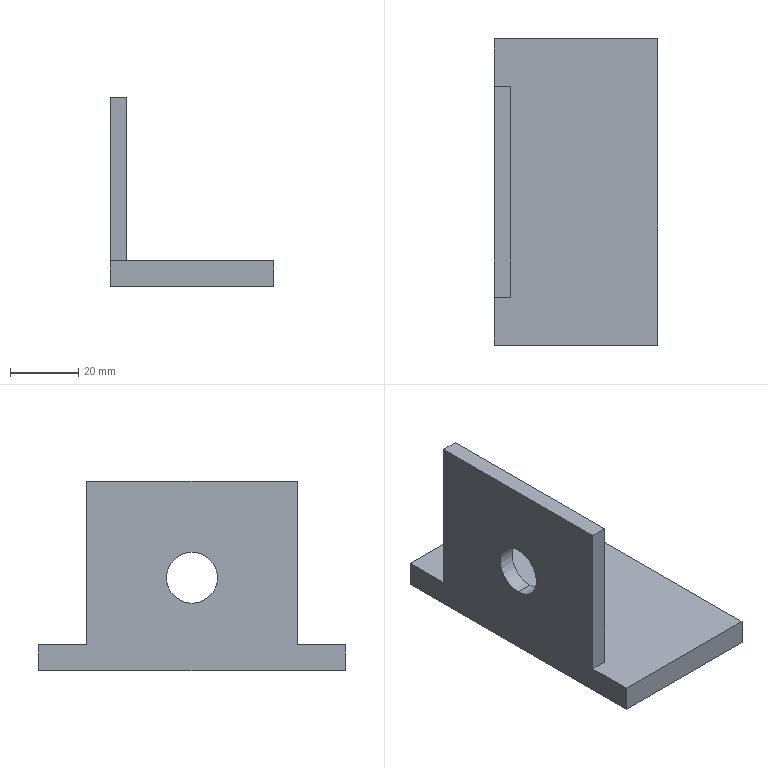Part | STEP file | 1 solid | 12 faces | box 48 x 90 x 55.597 mm | volume 46408 mm3 | plane 10 | cylinder 2 | commonest cylinder face diameters 15 x2
STEP:
#1=CARTESIAN_POINT('',(0.,0.,0.));
#2=DIRECTION('',(0.,0.,1.));
#3=DIRECTION('',(1.,0.,0.));
#4=AXIS2_PLACEMENT_3D('',#1,#2,#3);
#5=CARTESIAN_POINT('',(-595.146,553.5,112.406));
#6=VERTEX_POINT('',#5);
#7=CARTESIAN_POINT('',(-600.,553.5,112.406));
#8=VERTEX_POINT('',#7);
#9=CARTESIAN_POINT('',(-542.,553.5,112.406));
#10=DIRECTION('',(-1.,0.,0.));
#11=VECTOR('',#10,1.);
#12=LINE('',#9,#11);
#13=CARTESIAN_POINT('',(-542.,553.5,104.906));
#14=DIRECTION('',(-1.,0.,0.));
#15=DIRECTION('',(0.,0.,1.));
#16=AXIS2_PLACEMENT_3D('',#13,#14,#15);
#17=CYLINDRICAL_SURFACE('',#16,7.5);
#18=CARTESIAN_POINT('',(6.283,0.));
#19=DIRECTION('',(0.,1.));
#20=VECTOR('',#19,1.);
#21=LINE('',#18,#20);
#22=(GEOMETRIC_REPRESENTATION_CONTEXT(2)PARAMETRIC_REPRESENTATION_CONTEXT()REPRESENTATION_CONTEXT('',''));
#23=DEFINITIONAL_REPRESENTATION('',(#21),#22);
#24=PCURVE('',#17,#23);
#25=CARTESIAN_POINT('',(-542.,553.5,104.906));
#26=DIRECTION('',(-1.,0.,0.));
#27=DIRECTION('',(0.,0.,1.));
#28=AXIS2_PLACEMENT_3D('',#25,#26,#27);
#29=CYLINDRICAL_SURFACE('',#28,7.5);
#30=CARTESIAN_POINT('',(0.,0.));
#31=DIRECTION('',(0.,1.));
#32=VECTOR('',#31,1.);
#33=LINE('',#30,#32);
#34=(GEOMETRIC_REPRESENTATION_CONTEXT(2)PARAMETRIC_REPRESENTATION_CONTEXT()REPRESENTATION_CONTEXT('',''));
#35=DEFINITIONAL_REPRESENTATION('',(#33),#34);
#36=PCURVE('',#29,#35);
#37=SURFACE_CURVE('',#12,(#24,#36),.PCURVE_S1.);
#38=EDGE_CURVE('',#6,#8,#37,.T.);
#39=ORIENTED_EDGE('',*,*,#38,.T.);
#40=CARTESIAN_POINT('',(-600.,553.5,97.406));
#41=VERTEX_POINT('',#40);
#42=CARTESIAN_POINT('',(-600.,553.5,104.906));
#43=DIRECTION('',(-1.,0.,0.));
#44=DIRECTION('',(0.,0.,1.));
#45=AXIS2_PLACEMENT_3D('',#42,#43,#44);
#46=CIRCLE('',#45,7.5);
#47=CARTESIAN_POINT('',(0.,58.));
#48=DIRECTION('',(1.,0.));
#49=VECTOR('',#48,1.);
#50=LINE('',#47,#49);
#51=(GEOMETRIC_REPRESENTATION_CONTEXT(2)PARAMETRIC_REPRESENTATION_CONTEXT()REPRESENTATION_CONTEXT('',''));
#52=DEFINITIONAL_REPRESENTATION('',(#50),#51);
#53=PCURVE('',#17,#52);
#54=CARTESIAN_POINT('',(-600.,0.,133.232));
#55=DIRECTION('',(1.,0.,0.));
#56=DIRECTION('',(0.,0.,-1.));
#57=AXIS2_PLACEMENT_3D('',#54,#55,#56);
#58=PLANE('',#57);
#59=CARTESIAN_POINT('',(20.826,553.5));
#60=CARTESIAN_POINT('',(20.826,566.49));
#61=CARTESIAN_POINT('',(32.076,559.995));
#62=CARTESIAN_POINT('',(43.326,553.5));
#63=CARTESIAN_POINT('',(32.076,547.005));
#64=CARTESIAN_POINT('',(20.826,540.51));
#65=CARTESIAN_POINT('',(20.826,553.5));
#66=(BOUNDED_CURVE()B_SPLINE_CURVE(2,(#59,#60,#61,#62,#63,#64,#65),.UNSPECIFIED.,.T.,.F.)B_SPLINE_CURVE_WITH_KNOTS((1,2,2,2,2,1),(-2.094,0.,2.094,4.189,6.283,8.378),.UNSPECIFIED.)CURVE()GEOMETRIC_REPRESENTATION_ITEM()RATIONAL_B_SPLINE_CURVE((1.,0.5,1.,0.5,1.,0.5,1.))REPRESENTATION_ITEM(''));
#67=(GEOMETRIC_REPRESENTATION_CONTEXT(2)PARAMETRIC_REPRESENTATION_CONTEXT()REPRESENTATION_CONTEXT('',''));
#68=DEFINITIONAL_REPRESENTATION('',(#66),#67);
#69=PCURVE('',#58,#68);
#70=SURFACE_CURVE('',#46,(#53,#69),.PCURVE_S1.);
#71=EDGE_CURVE('',#41,#8,#70,.T.);
#72=ORIENTED_EDGE('',*,*,#71,.F.);
#73=CARTESIAN_POINT('',(-595.146,553.5,97.406));
#74=VERTEX_POINT('',#73);
#75=CARTESIAN_POINT('',(-542.,553.5,97.406));
#76=DIRECTION('',(-1.,0.,0.));
#77=VECTOR('',#76,1.);
#78=LINE('',#75,#77);
#79=CARTESIAN_POINT('',(3.142,0.));
#80=DIRECTION('',(0.,1.));
#81=VECTOR('',#80,1.);
#82=LINE('',#79,#81);
#83=(GEOMETRIC_REPRESENTATION_CONTEXT(2)PARAMETRIC_REPRESENTATION_CONTEXT()REPRESENTATION_CONTEXT('',''));
#84=DEFINITIONAL_REPRESENTATION('',(#82),#83);
#85=PCURVE('',#17,#84);
#86=CARTESIAN_POINT('',(3.142,0.));
#87=DIRECTION('',(0.,1.));
#88=VECTOR('',#87,1.);
#89=LINE('',#86,#88);
#90=(GEOMETRIC_REPRESENTATION_CONTEXT(2)PARAMETRIC_REPRESENTATION_CONTEXT()REPRESENTATION_CONTEXT('',''));
#91=DEFINITIONAL_REPRESENTATION('',(#89),#90);
#92=PCURVE('',#29,#91);
#93=SURFACE_CURVE('',#78,(#85,#92),.PCURVE_S1.);
#94=EDGE_CURVE('',#74,#41,#93,.T.);
#95=ORIENTED_EDGE('',*,*,#94,.F.);
#96=CARTESIAN_POINT('',(-595.146,553.5,104.906));
#97=DIRECTION('',(-1.,0.,0.));
#98=DIRECTION('',(0.,0.,1.));
#99=AXIS2_PLACEMENT_3D('',#96,#97,#98);
#100=CIRCLE('',#99,7.5);
#101=CARTESIAN_POINT('',(0.,53.146));
#102=DIRECTION('',(1.,0.));
#103=VECTOR('',#102,1.);
#104=LINE('',#101,#103);
#105=(GEOMETRIC_REPRESENTATION_CONTEXT(2)PARAMETRIC_REPRESENTATION_CONTEXT()REPRESENTATION_CONTEXT('',''));
#106=DEFINITIONAL_REPRESENTATION('',(#104),#105);
#107=PCURVE('',#17,#106);
#108=CARTESIAN_POINT('',(-595.146,0.,133.232));
#109=DIRECTION('',(-1.,0.,0.));
#110=DIRECTION('',(0.,0.,1.));
#111=AXIS2_PLACEMENT_3D('',#108,#109,#110);
#112=PLANE('',#111);
#113=CARTESIAN_POINT('',(-28.326,553.5));
#114=DIRECTION('',(1.,0.));
#115=AXIS2_PLACEMENT_2D('',#113,#114);
#116=CIRCLE('',#115,7.5);
#117=(GEOMETRIC_REPRESENTATION_CONTEXT(2)PARAMETRIC_REPRESENTATION_CONTEXT()REPRESENTATION_CONTEXT('',''));
#118=DEFINITIONAL_REPRESENTATION('',(#116),#117);
#119=PCURVE('',#112,#118);
#120=SURFACE_CURVE('',#100,(#107,#119),.PCURVE_S1.);
#121=EDGE_CURVE('',#74,#6,#120,.T.);
#122=ORIENTED_EDGE('',*,*,#121,.T.);
#123=EDGE_LOOP('',(#39,#72,#95,#122));
#124=FACE_BOUND('',#123,.F.);
#125=ADVANCED_FACE('',(#124),#17,.F.);
#126=CARTESIAN_POINT('',(-600.,553.5,104.906));
#127=DIRECTION('',(-1.,0.,0.));
#128=DIRECTION('',(0.,0.,1.));
#129=AXIS2_PLACEMENT_3D('',#126,#127,#128);
#130=CIRCLE('',#129,7.5);
#131=CARTESIAN_POINT('',(20.826,553.5));
#132=CARTESIAN_POINT('',(20.826,566.49));
#133=CARTESIAN_POINT('',(32.076,559.995));
#134=CARTESIAN_POINT('',(43.326,553.5));
#135=CARTESIAN_POINT('',(32.076,547.005));
#136=CARTESIAN_POINT('',(20.826,540.51));
#137=CARTESIAN_POINT('',(20.826,553.5));
#138=(BOUNDED_CURVE()B_SPLINE_CURVE(2,(#131,#132,#133,#134,#135,#136,#137),.UNSPECIFIED.,.T.,.F.)B_SPLINE_CURVE_WITH_KNOTS((1,2,2,2,2,1),(-2.094,0.,2.094,4.189,6.283,8.378),.UNSPECIFIED.)CURVE()GEOMETRIC_REPRESENTATION_ITEM()RATIONAL_B_SPLINE_CURVE((1.,0.5,1.,0.5,1.,0.5,1.))REPRESENTATION_ITEM(''));
#139=(GEOMETRIC_REPRESENTATION_CONTEXT(2)PARAMETRIC_REPRESENTATION_CONTEXT()REPRESENTATION_CONTEXT('',''));
#140=DEFINITIONAL_REPRESENTATION('',(#138),#139);
#141=PCURVE('',#58,#140);
#142=CARTESIAN_POINT('',(0.,58.));
#143=DIRECTION('',(1.,0.));
#144=VECTOR('',#143,1.);
#145=LINE('',#142,#144);
#146=(GEOMETRIC_REPRESENTATION_CONTEXT(2)PARAMETRIC_REPRESENTATION_CONTEXT()REPRESENTATION_CONTEXT('',''));
#147=DEFINITIONAL_REPRESENTATION('',(#145),#146);
#148=PCURVE('',#29,#147);
#149=SURFACE_CURVE('',#130,(#141,#148),.PCURVE_S1.);
#150=EDGE_CURVE('',#8,#41,#149,.T.);
#151=ORIENTED_EDGE('',*,*,#150,.F.);
#152=ORIENTED_EDGE('',*,*,#71,.F.);
#153=EDGE_LOOP('',(#151,#152));
#154=FACE_BOUND('',#153,.T.);
#155=CARTESIAN_POINT('',(-600.,584.5,133.232));
#156=VERTEX_POINT('',#155);
#157=CARTESIAN_POINT('',(-600.,522.5,133.232));
#158=VERTEX_POINT('',#157);
#159=CARTESIAN_POINT('',(-600.,0.,133.232));
#160=DIRECTION('',(0.,-1.,0.));
#161=VECTOR('',#160,1.);
#162=LINE('',#159,#161);
#163=CARTESIAN_POINT('',(0.,0.));
#164=DIRECTION('',(0.,-1.));
#165=VECTOR('',#164,1.);
#166=LINE('',#163,#165);
#167=(GEOMETRIC_REPRESENTATION_CONTEXT(2)PARAMETRIC_REPRESENTATION_CONTEXT()REPRESENTATION_CONTEXT('',''));
#168=DEFINITIONAL_REPRESENTATION('',(#166),#167);
#169=PCURVE('',#58,#168);
#170=CARTESIAN_POINT('',(0.,0.,133.232));
#171=DIRECTION('',(0.,0.,1.));
#172=DIRECTION('',(1.,0.,0.));
#173=AXIS2_PLACEMENT_3D('',#170,#171,#172);
#174=PLANE('',#173);
#175=CARTESIAN_POINT('',(-600.,0.));
#176=DIRECTION('',(0.,-1.));
#177=VECTOR('',#176,1.);
#178=LINE('',#175,#177);
#179=(GEOMETRIC_REPRESENTATION_CONTEXT(2)PARAMETRIC_REPRESENTATION_CONTEXT()REPRESENTATION_CONTEXT('',''));
#180=DEFINITIONAL_REPRESENTATION('',(#178),#179);
#181=PCURVE('',#174,#180);
#182=SURFACE_CURVE('',#162,(#169,#181),.PCURVE_S1.);
#183=EDGE_CURVE('',#156,#158,#182,.T.);
#184=ORIENTED_EDGE('',*,*,#183,.F.);
#185=CARTESIAN_POINT('',(-600.,584.5,85.232));
#186=VERTEX_POINT('',#185);
#187=CARTESIAN_POINT('',(-600.,584.5,133.232));
#188=DIRECTION('',(0.,0.,-1.));
#189=VECTOR('',#188,1.);
#190=LINE('',#187,#189);
#191=CARTESIAN_POINT('',(0.,584.5));
#192=DIRECTION('',(1.,0.));
#193=VECTOR('',#192,1.);
#194=LINE('',#191,#193);
#195=(GEOMETRIC_REPRESENTATION_CONTEXT(2)PARAMETRIC_REPRESENTATION_CONTEXT()REPRESENTATION_CONTEXT('',''));
#196=DEFINITIONAL_REPRESENTATION('',(#194),#195);
#197=PCURVE('',#58,#196);
#198=CARTESIAN_POINT('',(-648.717,584.5,133.232));
#199=DIRECTION('',(0.,1.,0.));
#200=DIRECTION('',(0.,0.,1.));
#201=AXIS2_PLACEMENT_3D('',#198,#199,#200);
#202=PLANE('',#201);
#203=CARTESIAN_POINT('',(0.,48.717));
#204=DIRECTION('',(-1.,0.));
#205=VECTOR('',#204,1.);
#206=LINE('',#203,#205);
#207=(GEOMETRIC_REPRESENTATION_CONTEXT(2)PARAMETRIC_REPRESENTATION_CONTEXT()REPRESENTATION_CONTEXT('',''));
#208=DEFINITIONAL_REPRESENTATION('',(#206),#207);
#209=PCURVE('',#202,#208);
#210=SURFACE_CURVE('',#190,(#197,#209),.PCURVE_S1.);
#211=EDGE_CURVE('',#156,#186,#210,.T.);
#212=ORIENTED_EDGE('',*,*,#211,.T.);
#213=CARTESIAN_POINT('',(-600.,598.5,85.232));
#214=VERTEX_POINT('',#213);
#215=CARTESIAN_POINT('',(-600.,0.,85.232));
#216=DIRECTION('',(0.,1.,0.));
#217=VECTOR('',#216,1.);
#218=LINE('',#215,#217);
#219=CARTESIAN_POINT('',(48.,0.));
#220=DIRECTION('',(0.,1.));
#221=VECTOR('',#220,1.);
#222=LINE('',#219,#221);
#223=(GEOMETRIC_REPRESENTATION_CONTEXT(2)PARAMETRIC_REPRESENTATION_CONTEXT()REPRESENTATION_CONTEXT('',''));
#224=DEFINITIONAL_REPRESENTATION('',(#222),#223);
#225=PCURVE('',#58,#224);
#226=CARTESIAN_POINT('',(-552.,0.,85.232));
#227=DIRECTION('',(0.,0.,1.));
#228=DIRECTION('',(1.,0.,0.));
#229=AXIS2_PLACEMENT_3D('',#226,#227,#228);
#230=PLANE('',#229);
#231=CARTESIAN_POINT('',(-48.,0.));
#232=DIRECTION('',(0.,1.));
#233=VECTOR('',#232,1.);
#234=LINE('',#231,#233);
#235=(GEOMETRIC_REPRESENTATION_CONTEXT(2)PARAMETRIC_REPRESENTATION_CONTEXT()REPRESENTATION_CONTEXT('',''));
#236=DEFINITIONAL_REPRESENTATION('',(#234),#235);
#237=PCURVE('',#230,#236);
#238=SURFACE_CURVE('',#218,(#225,#237),.PCURVE_S1.);
#239=EDGE_CURVE('',#186,#214,#238,.T.);
#240=ORIENTED_EDGE('',*,*,#239,.T.);
#241=CARTESIAN_POINT('',(-600.,598.5,77.635));
#242=VERTEX_POINT('',#241);
#243=CARTESIAN_POINT('',(-600.,598.5,0.));
#244=DIRECTION('',(0.,0.,1.));
#245=VECTOR('',#244,1.);
#246=LINE('',#243,#245);
#247=CARTESIAN_POINT('',(133.232,598.5));
#248=DIRECTION('',(-1.,0.));
#249=VECTOR('',#248,1.);
#250=LINE('',#247,#249);
#251=(GEOMETRIC_REPRESENTATION_CONTEXT(2)PARAMETRIC_REPRESENTATION_CONTEXT()REPRESENTATION_CONTEXT('',''));
#252=DEFINITIONAL_REPRESENTATION('',(#250),#251);
#253=PCURVE('',#58,#252);
#254=CARTESIAN_POINT('',(-552.,598.5,0.));
#255=DIRECTION('',(0.,-1.,0.));
#256=DIRECTION('',(0.,0.,-1.));
#257=AXIS2_PLACEMENT_3D('',#254,#255,#256);
#258=PLANE('',#257);
#259=CARTESIAN_POINT('',(0.,-48.));
#260=DIRECTION('',(-1.,0.));
#261=VECTOR('',#260,1.);
#262=LINE('',#259,#261);
#263=(GEOMETRIC_REPRESENTATION_CONTEXT(2)PARAMETRIC_REPRESENTATION_CONTEXT()REPRESENTATION_CONTEXT('',''));
#264=DEFINITIONAL_REPRESENTATION('',(#262),#263);
#265=PCURVE('',#258,#264);
#266=SURFACE_CURVE('',#246,(#253,#265),.PCURVE_S1.);
#267=EDGE_CURVE('',#242,#214,#266,.T.);
#268=ORIENTED_EDGE('',*,*,#267,.F.);
#269=CARTESIAN_POINT('',(-600.,508.5,77.635));
#270=VERTEX_POINT('',#269);
#271=CARTESIAN_POINT('',(-600.,0.,77.635));
#272=DIRECTION('',(0.,1.,0.));
#273=VECTOR('',#272,1.);
#274=LINE('',#271,#273);
#275=CARTESIAN_POINT('',(55.597,0.));
#276=DIRECTION('',(0.,1.));
#277=VECTOR('',#276,1.);
#278=LINE('',#275,#277);
#279=(GEOMETRIC_REPRESENTATION_CONTEXT(2)PARAMETRIC_REPRESENTATION_CONTEXT()REPRESENTATION_CONTEXT('',''));
#280=DEFINITIONAL_REPRESENTATION('',(#278),#279);
#281=PCURVE('',#58,#280);
#282=CARTESIAN_POINT('',(-552.,0.,77.635));
#283=DIRECTION('',(0.,0.,1.));
#284=DIRECTION('',(1.,0.,0.));
#285=AXIS2_PLACEMENT_3D('',#282,#283,#284);
#286=PLANE('',#285);
#287=CARTESIAN_POINT('',(-48.,0.));
#288=DIRECTION('',(0.,1.));
#289=VECTOR('',#288,1.);
#290=LINE('',#287,#289);
#291=(GEOMETRIC_REPRESENTATION_CONTEXT(2)PARAMETRIC_REPRESENTATION_CONTEXT()REPRESENTATION_CONTEXT('',''));
#292=DEFINITIONAL_REPRESENTATION('',(#290),#291);
#293=PCURVE('',#286,#292);
#294=SURFACE_CURVE('',#274,(#281,#293),.PCURVE_S1.);
#295=EDGE_CURVE('',#270,#242,#294,.T.);
#296=ORIENTED_EDGE('',*,*,#295,.F.);
#297=CARTESIAN_POINT('',(-600.,508.5,85.232));
#298=VERTEX_POINT('',#297);
#299=CARTESIAN_POINT('',(-600.,508.5,0.));
#300=DIRECTION('',(0.,0.,1.));
#301=VECTOR('',#300,1.);
#302=LINE('',#299,#301);
#303=CARTESIAN_POINT('',(133.232,508.5));
#304=DIRECTION('',(-1.,0.));
#305=VECTOR('',#304,1.);
#306=LINE('',#303,#305);
#307=(GEOMETRIC_REPRESENTATION_CONTEXT(2)PARAMETRIC_REPRESENTATION_CONTEXT()REPRESENTATION_CONTEXT('',''));
#308=DEFINITIONAL_REPRESENTATION('',(#306),#307);
#309=PCURVE('',#58,#308);
#310=CARTESIAN_POINT('',(-552.,508.5,0.));
#311=DIRECTION('',(0.,-1.,0.));
#312=DIRECTION('',(0.,0.,-1.));
#313=AXIS2_PLACEMENT_3D('',#310,#311,#312);
#314=PLANE('',#313);
#315=CARTESIAN_POINT('',(0.,-48.));
#316=DIRECTION('',(-1.,0.));
#317=VECTOR('',#316,1.);
#318=LINE('',#315,#317);
#319=(GEOMETRIC_REPRESENTATION_CONTEXT(2)PARAMETRIC_REPRESENTATION_CONTEXT()REPRESENTATION_CONTEXT('',''));
#320=DEFINITIONAL_REPRESENTATION('',(#318),#319);
#321=PCURVE('',#314,#320);
#322=SURFACE_CURVE('',#302,(#309,#321),.PCURVE_S1.);
#323=EDGE_CURVE('',#270,#298,#322,.T.);
#324=ORIENTED_EDGE('',*,*,#323,.T.);
#325=CARTESIAN_POINT('',(-600.,522.5,85.232));
#326=VERTEX_POINT('',#325);
#327=CARTESIAN_POINT('',(-600.,0.,85.232));
#328=DIRECTION('',(0.,1.,0.));
#329=VECTOR('',#328,1.);
#330=LINE('',#327,#329);
#331=CARTESIAN_POINT('',(48.,0.));
#332=DIRECTION('',(0.,1.));
#333=VECTOR('',#332,1.);
#334=LINE('',#331,#333);
#335=(GEOMETRIC_REPRESENTATION_CONTEXT(2)PARAMETRIC_REPRESENTATION_CONTEXT()REPRESENTATION_CONTEXT('',''));
#336=DEFINITIONAL_REPRESENTATION('',(#334),#335);
#337=PCURVE('',#58,#336);
#338=CARTESIAN_POINT('',(-48.,0.));
#339=DIRECTION('',(0.,1.));
#340=VECTOR('',#339,1.);
#341=LINE('',#338,#340);
#342=(GEOMETRIC_REPRESENTATION_CONTEXT(2)PARAMETRIC_REPRESENTATION_CONTEXT()REPRESENTATION_CONTEXT('',''));
#343=DEFINITIONAL_REPRESENTATION('',(#341),#342);
#344=PCURVE('',#230,#343);
#345=SURFACE_CURVE('',#330,(#337,#344),.PCURVE_S1.);
#346=EDGE_CURVE('',#298,#326,#345,.T.);
#347=ORIENTED_EDGE('',*,*,#346,.T.);
#348=CARTESIAN_POINT('',(-600.,522.5,133.232));
#349=DIRECTION('',(0.,0.,1.));
#350=VECTOR('',#349,1.);
#351=LINE('',#348,#350);
#352=CARTESIAN_POINT('',(0.,522.5));
#353=DIRECTION('',(-1.,0.));
#354=VECTOR('',#353,1.);
#355=LINE('',#352,#354);
#356=(GEOMETRIC_REPRESENTATION_CONTEXT(2)PARAMETRIC_REPRESENTATION_CONTEXT()REPRESENTATION_CONTEXT('',''));
#357=DEFINITIONAL_REPRESENTATION('',(#355),#356);
#358=PCURVE('',#58,#357);
#359=CARTESIAN_POINT('',(-648.717,522.5,133.232));
#360=DIRECTION('',(0.,-1.,0.));
#361=DIRECTION('',(0.,0.,-1.));
#362=AXIS2_PLACEMENT_3D('',#359,#360,#361);
#363=PLANE('',#362);
#364=CARTESIAN_POINT('',(0.,48.717));
#365=DIRECTION('',(-1.,0.));
#366=VECTOR('',#365,1.);
#367=LINE('',#364,#366);
#368=(GEOMETRIC_REPRESENTATION_CONTEXT(2)PARAMETRIC_REPRESENTATION_CONTEXT()REPRESENTATION_CONTEXT('',''));
#369=DEFINITIONAL_REPRESENTATION('',(#367),#368);
#370=PCURVE('',#363,#369);
#371=SURFACE_CURVE('',#351,(#358,#370),.PCURVE_S1.);
#372=EDGE_CURVE('',#326,#158,#371,.T.);
#373=ORIENTED_EDGE('',*,*,#372,.T.);
#374=EDGE_LOOP('',(#184,#212,#240,#268,#296,#324,#347,#373));
#375=FACE_BOUND('',#374,.T.);
#376=ADVANCED_FACE('',(#154,#375),#58,.F.);
#377=CARTESIAN_POINT('',(-595.146,553.5,104.906));
#378=DIRECTION('',(-1.,0.,0.));
#379=DIRECTION('',(0.,0.,1.));
#380=AXIS2_PLACEMENT_3D('',#377,#378,#379);
#381=CIRCLE('',#380,7.5);
#382=CARTESIAN_POINT('',(-28.326,553.5));
#383=DIRECTION('',(1.,0.));
#384=AXIS2_PLACEMENT_2D('',#382,#383);
#385=CIRCLE('',#384,7.5);
#386=(GEOMETRIC_REPRESENTATION_CONTEXT(2)PARAMETRIC_REPRESENTATION_CONTEXT()REPRESENTATION_CONTEXT('',''));
#387=DEFINITIONAL_REPRESENTATION('',(#385),#386);
#388=PCURVE('',#112,#387);
#389=CARTESIAN_POINT('',(0.,53.146));
#390=DIRECTION('',(1.,0.));
#391=VECTOR('',#390,1.);
#392=LINE('',#389,#391);
#393=(GEOMETRIC_REPRESENTATION_CONTEXT(2)PARAMETRIC_REPRESENTATION_CONTEXT()REPRESENTATION_CONTEXT('',''));
#394=DEFINITIONAL_REPRESENTATION('',(#392),#393);
#395=PCURVE('',#29,#394);
#396=SURFACE_CURVE('',#381,(#388,#395),.PCURVE_S1.);
#397=EDGE_CURVE('',#6,#74,#396,.T.);
#398=ORIENTED_EDGE('',*,*,#397,.T.);
#399=ORIENTED_EDGE('',*,*,#121,.T.);
#400=EDGE_LOOP('',(#398,#399));
#401=FACE_BOUND('',#400,.T.);
#402=CARTESIAN_POINT('',(-595.146,522.5,85.232));
#403=VERTEX_POINT('',#402);
#404=CARTESIAN_POINT('',(-595.146,584.5,85.232));
#405=VERTEX_POINT('',#404);
#406=CARTESIAN_POINT('',(-595.146,0.,85.232));
#407=DIRECTION('',(0.,1.,0.));
#408=VECTOR('',#407,1.);
#409=LINE('',#406,#408);
#410=CARTESIAN_POINT('',(-48.,0.));
#411=DIRECTION('',(0.,1.));
#412=VECTOR('',#411,1.);
#413=LINE('',#410,#412);
#414=(GEOMETRIC_REPRESENTATION_CONTEXT(2)PARAMETRIC_REPRESENTATION_CONTEXT()REPRESENTATION_CONTEXT('',''));
#415=DEFINITIONAL_REPRESENTATION('',(#413),#414);
#416=PCURVE('',#112,#415);
#417=CARTESIAN_POINT('',(-43.146,0.));
#418=DIRECTION('',(0.,1.));
#419=VECTOR('',#418,1.);
#420=LINE('',#417,#419);
#421=(GEOMETRIC_REPRESENTATION_CONTEXT(2)PARAMETRIC_REPRESENTATION_CONTEXT()REPRESENTATION_CONTEXT('',''));
#422=DEFINITIONAL_REPRESENTATION('',(#420),#421);
#423=PCURVE('',#230,#422);
#424=SURFACE_CURVE('',#409,(#416,#423),.PCURVE_S1.);
#425=EDGE_CURVE('',#403,#405,#424,.T.);
#426=ORIENTED_EDGE('',*,*,#425,.T.);
#427=CARTESIAN_POINT('',(-595.146,584.5,133.232));
#428=VERTEX_POINT('',#427);
#429=CARTESIAN_POINT('',(-595.146,584.5,133.232));
#430=DIRECTION('',(0.,0.,1.));
#431=VECTOR('',#430,1.);
#432=LINE('',#429,#431);
#433=CARTESIAN_POINT('',(0.,584.5));
#434=DIRECTION('',(1.,0.));
#435=VECTOR('',#434,1.);
#436=LINE('',#433,#435);
#437=(GEOMETRIC_REPRESENTATION_CONTEXT(2)PARAMETRIC_REPRESENTATION_CONTEXT()REPRESENTATION_CONTEXT('',''));
#438=DEFINITIONAL_REPRESENTATION('',(#436),#437);
#439=PCURVE('',#112,#438);
#440=CARTESIAN_POINT('',(0.,53.571));
#441=DIRECTION('',(1.,0.));
#442=VECTOR('',#441,1.);
#443=LINE('',#440,#442);
#444=(GEOMETRIC_REPRESENTATION_CONTEXT(2)PARAMETRIC_REPRESENTATION_CONTEXT()REPRESENTATION_CONTEXT('',''));
#445=DEFINITIONAL_REPRESENTATION('',(#443),#444);
#446=PCURVE('',#202,#445);
#447=SURFACE_CURVE('',#432,(#439,#446),.PCURVE_S1.);
#448=EDGE_CURVE('',#405,#428,#447,.T.);
#449=ORIENTED_EDGE('',*,*,#448,.T.);
#450=CARTESIAN_POINT('',(-595.146,522.5,133.232));
#451=VERTEX_POINT('',#450);
#452=CARTESIAN_POINT('',(-595.146,0.,133.232));
#453=DIRECTION('',(0.,1.,0.));
#454=VECTOR('',#453,1.);
#455=LINE('',#452,#454);
#456=CARTESIAN_POINT('',(0.,0.));
#457=DIRECTION('',(0.,1.));
#458=VECTOR('',#457,1.);
#459=LINE('',#456,#458);
#460=(GEOMETRIC_REPRESENTATION_CONTEXT(2)PARAMETRIC_REPRESENTATION_CONTEXT()REPRESENTATION_CONTEXT('',''));
#461=DEFINITIONAL_REPRESENTATION('',(#459),#460);
#462=PCURVE('',#112,#461);
#463=CARTESIAN_POINT('',(-595.146,0.));
#464=DIRECTION('',(0.,1.));
#465=VECTOR('',#464,1.);
#466=LINE('',#463,#465);
#467=(GEOMETRIC_REPRESENTATION_CONTEXT(2)PARAMETRIC_REPRESENTATION_CONTEXT()REPRESENTATION_CONTEXT('',''));
#468=DEFINITIONAL_REPRESENTATION('',(#466),#467);
#469=PCURVE('',#174,#468);
#470=SURFACE_CURVE('',#455,(#462,#469),.PCURVE_S1.);
#471=EDGE_CURVE('',#451,#428,#470,.T.);
#472=ORIENTED_EDGE('',*,*,#471,.F.);
#473=CARTESIAN_POINT('',(-595.146,522.5,133.232));
#474=DIRECTION('',(0.,0.,-1.));
#475=VECTOR('',#474,1.);
#476=LINE('',#473,#475);
#477=CARTESIAN_POINT('',(0.,522.5));
#478=DIRECTION('',(-1.,0.));
#479=VECTOR('',#478,1.);
#480=LINE('',#477,#479);
#481=(GEOMETRIC_REPRESENTATION_CONTEXT(2)PARAMETRIC_REPRESENTATION_CONTEXT()REPRESENTATION_CONTEXT('',''));
#482=DEFINITIONAL_REPRESENTATION('',(#480),#481);
#483=PCURVE('',#112,#482);
#484=CARTESIAN_POINT('',(0.,53.571));
#485=DIRECTION('',(1.,0.));
#486=VECTOR('',#485,1.);
#487=LINE('',#484,#486);
#488=(GEOMETRIC_REPRESENTATION_CONTEXT(2)PARAMETRIC_REPRESENTATION_CONTEXT()REPRESENTATION_CONTEXT('',''));
#489=DEFINITIONAL_REPRESENTATION('',(#487),#488);
#490=PCURVE('',#363,#489);
#491=SURFACE_CURVE('',#476,(#483,#490),.PCURVE_S1.);
#492=EDGE_CURVE('',#451,#403,#491,.T.);
#493=ORIENTED_EDGE('',*,*,#492,.T.);
#494=EDGE_LOOP('',(#426,#449,#472,#493));
#495=FACE_BOUND('',#494,.T.);
#496=ADVANCED_FACE('',(#401,#495),#112,.F.);
#497=ORIENTED_EDGE('',*,*,#183,.T.);
#498=CARTESIAN_POINT('',(-648.717,522.5,133.232));
#499=DIRECTION('',(1.,0.,0.));
#500=VECTOR('',#499,1.);
#501=LINE('',#498,#500);
#502=CARTESIAN_POINT('',(-648.717,522.5));
#503=DIRECTION('',(1.,0.));
#504=VECTOR('',#503,1.);
#505=LINE('',#502,#504);
#506=(GEOMETRIC_REPRESENTATION_CONTEXT(2)PARAMETRIC_REPRESENTATION_CONTEXT()REPRESENTATION_CONTEXT('',''));
#507=DEFINITIONAL_REPRESENTATION('',(#505),#506);
#508=PCURVE('',#174,#507);
#509=CARTESIAN_POINT('',(0.,0.));
#510=DIRECTION('',(0.,1.));
#511=VECTOR('',#510,1.);
#512=LINE('',#509,#511);
#513=(GEOMETRIC_REPRESENTATION_CONTEXT(2)PARAMETRIC_REPRESENTATION_CONTEXT()REPRESENTATION_CONTEXT('',''));
#514=DEFINITIONAL_REPRESENTATION('',(#512),#513);
#515=PCURVE('',#363,#514);
#516=SURFACE_CURVE('',#501,(#508,#515),.PCURVE_S1.);
#517=EDGE_CURVE('',#158,#451,#516,.T.);
#518=ORIENTED_EDGE('',*,*,#517,.T.);
#519=ORIENTED_EDGE('',*,*,#471,.T.);
#520=CARTESIAN_POINT('',(-648.717,584.5,133.232));
#521=DIRECTION('',(1.,0.,0.));
#522=VECTOR('',#521,1.);
#523=LINE('',#520,#522);
#524=CARTESIAN_POINT('',(-648.717,584.5));
#525=DIRECTION('',(1.,0.));
#526=VECTOR('',#525,1.);
#527=LINE('',#524,#526);
#528=(GEOMETRIC_REPRESENTATION_CONTEXT(2)PARAMETRIC_REPRESENTATION_CONTEXT()REPRESENTATION_CONTEXT('',''));
#529=DEFINITIONAL_REPRESENTATION('',(#527),#528);
#530=PCURVE('',#174,#529);
#531=CARTESIAN_POINT('',(0.,0.));
#532=DIRECTION('',(0.,1.));
#533=VECTOR('',#532,1.);
#534=LINE('',#531,#533);
#535=(GEOMETRIC_REPRESENTATION_CONTEXT(2)PARAMETRIC_REPRESENTATION_CONTEXT()REPRESENTATION_CONTEXT('',''));
#536=DEFINITIONAL_REPRESENTATION('',(#534),#535);
#537=PCURVE('',#202,#536);
#538=SURFACE_CURVE('',#523,(#530,#537),.PCURVE_S1.);
#539=EDGE_CURVE('',#156,#428,#538,.T.);
#540=ORIENTED_EDGE('',*,*,#539,.F.);
#541=EDGE_LOOP('',(#497,#518,#519,#540));
#542=FACE_BOUND('',#541,.T.);
#543=ADVANCED_FACE('',(#542),#174,.T.);
#544=ORIENTED_EDGE('',*,*,#295,.T.);
#545=CARTESIAN_POINT('',(-552.,598.5,77.635));
#546=VERTEX_POINT('',#545);
#547=CARTESIAN_POINT('',(-552.,598.5,77.635));
#548=DIRECTION('',(-1.,0.,0.));
#549=VECTOR('',#548,1.);
#550=LINE('',#547,#549);
#551=CARTESIAN_POINT('',(0.,598.5));
#552=DIRECTION('',(-1.,0.));
#553=VECTOR('',#552,1.);
#554=LINE('',#551,#553);
#555=(GEOMETRIC_REPRESENTATION_CONTEXT(2)PARAMETRIC_REPRESENTATION_CONTEXT()REPRESENTATION_CONTEXT('',''));
#556=DEFINITIONAL_REPRESENTATION('',(#554),#555);
#557=PCURVE('',#286,#556);
#558=CARTESIAN_POINT('',(-77.635,0.));
#559=DIRECTION('',(0.,-1.));
#560=VECTOR('',#559,1.);
#561=LINE('',#558,#560);
#562=(GEOMETRIC_REPRESENTATION_CONTEXT(2)PARAMETRIC_REPRESENTATION_CONTEXT()REPRESENTATION_CONTEXT('',''));
#563=DEFINITIONAL_REPRESENTATION('',(#561),#562);
#564=PCURVE('',#258,#563);
#565=SURFACE_CURVE('',#550,(#557,#564),.PCURVE_S1.);
#566=EDGE_CURVE('',#546,#242,#565,.T.);
#567=ORIENTED_EDGE('',*,*,#566,.F.);
#568=CARTESIAN_POINT('',(-552.,508.5,77.635));
#569=VERTEX_POINT('',#568);
#570=CARTESIAN_POINT('',(-552.,0.,77.635));
#571=DIRECTION('',(0.,1.,0.));
#572=VECTOR('',#571,1.);
#573=LINE('',#570,#572);
#574=CARTESIAN_POINT('',(0.,0.));
#575=DIRECTION('',(0.,1.));
#576=VECTOR('',#575,1.);
#577=LINE('',#574,#576);
#578=(GEOMETRIC_REPRESENTATION_CONTEXT(2)PARAMETRIC_REPRESENTATION_CONTEXT()REPRESENTATION_CONTEXT('',''));
#579=DEFINITIONAL_REPRESENTATION('',(#577),#578);
#580=PCURVE('',#286,#579);
#581=CARTESIAN_POINT('',(-552.,0.,0.));
#582=DIRECTION('',(-1.,0.,0.));
#583=DIRECTION('',(0.,0.,1.));
#584=AXIS2_PLACEMENT_3D('',#581,#582,#583);
#585=PLANE('',#584);
#586=CARTESIAN_POINT('',(77.635,0.));
#587=DIRECTION('',(0.,1.));
#588=VECTOR('',#587,1.);
#589=LINE('',#586,#588);
#590=(GEOMETRIC_REPRESENTATION_CONTEXT(2)PARAMETRIC_REPRESENTATION_CONTEXT()REPRESENTATION_CONTEXT('',''));
#591=DEFINITIONAL_REPRESENTATION('',(#589),#590);
#592=PCURVE('',#585,#591);
#593=SURFACE_CURVE('',#573,(#580,#592),.PCURVE_S1.);
#594=EDGE_CURVE('',#569,#546,#593,.T.);
#595=ORIENTED_EDGE('',*,*,#594,.F.);
#596=CARTESIAN_POINT('',(-552.,508.5,77.635));
#597=DIRECTION('',(-1.,0.,0.));
#598=VECTOR('',#597,1.);
#599=LINE('',#596,#598);
#600=CARTESIAN_POINT('',(0.,508.5));
#601=DIRECTION('',(-1.,0.));
#602=VECTOR('',#601,1.);
#603=LINE('',#600,#602);
#604=(GEOMETRIC_REPRESENTATION_CONTEXT(2)PARAMETRIC_REPRESENTATION_CONTEXT()REPRESENTATION_CONTEXT('',''));
#605=DEFINITIONAL_REPRESENTATION('',(#603),#604);
#606=PCURVE('',#286,#605);
#607=CARTESIAN_POINT('',(-77.635,0.));
#608=DIRECTION('',(0.,-1.));
#609=VECTOR('',#608,1.);
#610=LINE('',#607,#609);
#611=(GEOMETRIC_REPRESENTATION_CONTEXT(2)PARAMETRIC_REPRESENTATION_CONTEXT()REPRESENTATION_CONTEXT('',''));
#612=DEFINITIONAL_REPRESENTATION('',(#610),#611);
#613=PCURVE('',#314,#612);
#614=SURFACE_CURVE('',#599,(#606,#613),.PCURVE_S1.);
#615=EDGE_CURVE('',#569,#270,#614,.T.);
#616=ORIENTED_EDGE('',*,*,#615,.T.);
#617=EDGE_LOOP('',(#544,#567,#595,#616));
#618=FACE_BOUND('',#617,.T.);
#619=ADVANCED_FACE('',(#618),#286,.F.);
#620=ORIENTED_EDGE('',*,*,#267,.T.);
#621=CARTESIAN_POINT('',(-552.,598.5,85.232));
#622=VERTEX_POINT('',#621);
#623=CARTESIAN_POINT('',(-552.,598.5,85.232));
#624=DIRECTION('',(-1.,0.,0.));
#625=VECTOR('',#624,1.);
#626=LINE('',#623,#625);
#627=CARTESIAN_POINT('',(-85.232,0.));
#628=DIRECTION('',(0.,-1.));
#629=VECTOR('',#628,1.);
#630=LINE('',#627,#629);
#631=(GEOMETRIC_REPRESENTATION_CONTEXT(2)PARAMETRIC_REPRESENTATION_CONTEXT()REPRESENTATION_CONTEXT('',''));
#632=DEFINITIONAL_REPRESENTATION('',(#630),#631);
#633=PCURVE('',#258,#632);
#634=CARTESIAN_POINT('',(0.,598.5));
#635=DIRECTION('',(-1.,0.));
#636=VECTOR('',#635,1.);
#637=LINE('',#634,#636);
#638=(GEOMETRIC_REPRESENTATION_CONTEXT(2)PARAMETRIC_REPRESENTATION_CONTEXT()REPRESENTATION_CONTEXT('',''));
#639=DEFINITIONAL_REPRESENTATION('',(#637),#638);
#640=PCURVE('',#230,#639);
#641=SURFACE_CURVE('',#626,(#633,#640),.PCURVE_S1.);
#642=EDGE_CURVE('',#622,#214,#641,.T.);
#643=ORIENTED_EDGE('',*,*,#642,.F.);
#644=CARTESIAN_POINT('',(-552.,598.5,0.));
#645=DIRECTION('',(0.,0.,1.));
#646=VECTOR('',#645,1.);
#647=LINE('',#644,#646);
#648=CARTESIAN_POINT('',(0.,0.));
#649=DIRECTION('',(-1.,0.));
#650=VECTOR('',#649,1.);
#651=LINE('',#648,#650);
#652=(GEOMETRIC_REPRESENTATION_CONTEXT(2)PARAMETRIC_REPRESENTATION_CONTEXT()REPRESENTATION_CONTEXT('',''));
#653=DEFINITIONAL_REPRESENTATION('',(#651),#652);
#654=PCURVE('',#258,#653);
#655=CARTESIAN_POINT('',(0.,598.5));
#656=DIRECTION('',(1.,0.));
#657=VECTOR('',#656,1.);
#658=LINE('',#655,#657);
#659=(GEOMETRIC_REPRESENTATION_CONTEXT(2)PARAMETRIC_REPRESENTATION_CONTEXT()REPRESENTATION_CONTEXT('',''));
#660=DEFINITIONAL_REPRESENTATION('',(#658),#659);
#661=PCURVE('',#585,#660);
#662=SURFACE_CURVE('',#647,(#654,#661),.PCURVE_S1.);
#663=EDGE_CURVE('',#546,#622,#662,.T.);
#664=ORIENTED_EDGE('',*,*,#663,.F.);
#665=ORIENTED_EDGE('',*,*,#566,.T.);
#666=EDGE_LOOP('',(#620,#643,#664,#665));
#667=FACE_BOUND('',#666,.T.);
#668=ADVANCED_FACE('',(#667),#258,.F.);
#669=CARTESIAN_POINT('',(-648.717,584.5,85.232));
#670=DIRECTION('',(1.,0.,0.));
#671=VECTOR('',#670,1.);
#672=LINE('',#669,#671);
#673=CARTESIAN_POINT('',(-96.717,584.5));
#674=DIRECTION('',(1.,0.));
#675=VECTOR('',#674,1.);
#676=LINE('',#673,#675);
#677=(GEOMETRIC_REPRESENTATION_CONTEXT(2)PARAMETRIC_REPRESENTATION_CONTEXT()REPRESENTATION_CONTEXT('',''));
#678=DEFINITIONAL_REPRESENTATION('',(#676),#677);
#679=PCURVE('',#230,#678);
#680=CARTESIAN_POINT('',(-48.,0.));
#681=DIRECTION('',(0.,1.));
#682=VECTOR('',#681,1.);
#683=LINE('',#680,#682);
#684=(GEOMETRIC_REPRESENTATION_CONTEXT(2)PARAMETRIC_REPRESENTATION_CONTEXT()REPRESENTATION_CONTEXT('',''));
#685=DEFINITIONAL_REPRESENTATION('',(#683),#684);
#686=PCURVE('',#202,#685);
#687=SURFACE_CURVE('',#672,(#679,#686),.PCURVE_S1.);
#688=EDGE_CURVE('',#186,#405,#687,.T.);
#689=ORIENTED_EDGE('',*,*,#688,.T.);
#690=ORIENTED_EDGE('',*,*,#425,.F.);
#691=CARTESIAN_POINT('',(-648.717,522.5,85.232));
#692=DIRECTION('',(1.,0.,0.));
#693=VECTOR('',#692,1.);
#694=LINE('',#691,#693);
#695=CARTESIAN_POINT('',(-96.717,522.5));
#696=DIRECTION('',(1.,0.));
#697=VECTOR('',#696,1.);
#698=LINE('',#695,#697);
#699=(GEOMETRIC_REPRESENTATION_CONTEXT(2)PARAMETRIC_REPRESENTATION_CONTEXT()REPRESENTATION_CONTEXT('',''));
#700=DEFINITIONAL_REPRESENTATION('',(#698),#699);
#701=PCURVE('',#230,#700);
#702=CARTESIAN_POINT('',(48.,0.));
#703=DIRECTION('',(0.,1.));
#704=VECTOR('',#703,1.);
#705=LINE('',#702,#704);
#706=(GEOMETRIC_REPRESENTATION_CONTEXT(2)PARAMETRIC_REPRESENTATION_CONTEXT()REPRESENTATION_CONTEXT('',''));
#707=DEFINITIONAL_REPRESENTATION('',(#705),#706);
#708=PCURVE('',#363,#707);
#709=SURFACE_CURVE('',#694,(#701,#708),.PCURVE_S1.);
#710=EDGE_CURVE('',#326,#403,#709,.T.);
#711=ORIENTED_EDGE('',*,*,#710,.F.);
#712=ORIENTED_EDGE('',*,*,#346,.F.);
#713=CARTESIAN_POINT('',(-552.,508.5,85.232));
#714=VERTEX_POINT('',#713);
#715=CARTESIAN_POINT('',(-552.,508.5,85.232));
#716=DIRECTION('',(-1.,0.,0.));
#717=VECTOR('',#716,1.);
#718=LINE('',#715,#717);
#719=CARTESIAN_POINT('',(0.,508.5));
#720=DIRECTION('',(-1.,0.));
#721=VECTOR('',#720,1.);
#722=LINE('',#719,#721);
#723=(GEOMETRIC_REPRESENTATION_CONTEXT(2)PARAMETRIC_REPRESENTATION_CONTEXT()REPRESENTATION_CONTEXT('',''));
#724=DEFINITIONAL_REPRESENTATION('',(#722),#723);
#725=PCURVE('',#230,#724);
#726=CARTESIAN_POINT('',(-85.232,0.));
#727=DIRECTION('',(0.,-1.));
#728=VECTOR('',#727,1.);
#729=LINE('',#726,#728);
#730=(GEOMETRIC_REPRESENTATION_CONTEXT(2)PARAMETRIC_REPRESENTATION_CONTEXT()REPRESENTATION_CONTEXT('',''));
#731=DEFINITIONAL_REPRESENTATION('',(#729),#730);
#732=PCURVE('',#314,#731);
#733=SURFACE_CURVE('',#718,(#725,#732),.PCURVE_S1.);
#734=EDGE_CURVE('',#714,#298,#733,.T.);
#735=ORIENTED_EDGE('',*,*,#734,.F.);
#736=CARTESIAN_POINT('',(-552.,0.,85.232));
#737=DIRECTION('',(0.,1.,0.));
#738=VECTOR('',#737,1.);
#739=LINE('',#736,#738);
#740=CARTESIAN_POINT('',(0.,0.));
#741=DIRECTION('',(0.,1.));
#742=VECTOR('',#741,1.);
#743=LINE('',#740,#742);
#744=(GEOMETRIC_REPRESENTATION_CONTEXT(2)PARAMETRIC_REPRESENTATION_CONTEXT()REPRESENTATION_CONTEXT('',''));
#745=DEFINITIONAL_REPRESENTATION('',(#743),#744);
#746=PCURVE('',#230,#745);
#747=CARTESIAN_POINT('',(85.232,0.));
#748=DIRECTION('',(0.,1.));
#749=VECTOR('',#748,1.);
#750=LINE('',#747,#749);
#751=(GEOMETRIC_REPRESENTATION_CONTEXT(2)PARAMETRIC_REPRESENTATION_CONTEXT()REPRESENTATION_CONTEXT('',''));
#752=DEFINITIONAL_REPRESENTATION('',(#750),#751);
#753=PCURVE('',#585,#752);
#754=SURFACE_CURVE('',#739,(#746,#753),.PCURVE_S1.);
#755=EDGE_CURVE('',#714,#622,#754,.T.);
#756=ORIENTED_EDGE('',*,*,#755,.T.);
#757=ORIENTED_EDGE('',*,*,#642,.T.);
#758=ORIENTED_EDGE('',*,*,#239,.F.);
#759=EDGE_LOOP('',(#689,#690,#711,#712,#735,#756,#757,#758));
#760=FACE_BOUND('',#759,.T.);
#761=ADVANCED_FACE('',(#760),#230,.T.);
#762=ORIENTED_EDGE('',*,*,#323,.F.);
#763=ORIENTED_EDGE('',*,*,#615,.F.);
#764=CARTESIAN_POINT('',(-552.,508.5,0.));
#765=DIRECTION('',(0.,0.,1.));
#766=VECTOR('',#765,1.);
#767=LINE('',#764,#766);
#768=CARTESIAN_POINT('',(0.,0.));
#769=DIRECTION('',(-1.,0.));
#770=VECTOR('',#769,1.);
#771=LINE('',#768,#770);
#772=(GEOMETRIC_REPRESENTATION_CONTEXT(2)PARAMETRIC_REPRESENTATION_CONTEXT()REPRESENTATION_CONTEXT('',''));
#773=DEFINITIONAL_REPRESENTATION('',(#771),#772);
#774=PCURVE('',#314,#773);
#775=CARTESIAN_POINT('',(0.,508.5));
#776=DIRECTION('',(1.,0.));
#777=VECTOR('',#776,1.);
#778=LINE('',#775,#777);
#779=(GEOMETRIC_REPRESENTATION_CONTEXT(2)PARAMETRIC_REPRESENTATION_CONTEXT()REPRESENTATION_CONTEXT('',''));
#780=DEFINITIONAL_REPRESENTATION('',(#778),#779);
#781=PCURVE('',#585,#780);
#782=SURFACE_CURVE('',#767,(#774,#781),.PCURVE_S1.);
#783=EDGE_CURVE('',#569,#714,#782,.T.);
#784=ORIENTED_EDGE('',*,*,#783,.T.);
#785=ORIENTED_EDGE('',*,*,#734,.T.);
#786=EDGE_LOOP('',(#762,#763,#784,#785));
#787=FACE_BOUND('',#786,.T.);
#788=ADVANCED_FACE('',(#787),#314,.T.);
#789=ORIENTED_EDGE('',*,*,#594,.T.);
#790=ORIENTED_EDGE('',*,*,#663,.T.);
#791=ORIENTED_EDGE('',*,*,#755,.F.);
#792=ORIENTED_EDGE('',*,*,#783,.F.);
#793=EDGE_LOOP('',(#789,#790,#791,#792));
#794=FACE_BOUND('',#793,.T.);
#795=ADVANCED_FACE('',(#794),#585,.F.);
#796=ORIENTED_EDGE('',*,*,#372,.F.);
#797=ORIENTED_EDGE('',*,*,#710,.T.);
#798=ORIENTED_EDGE('',*,*,#492,.F.);
#799=ORIENTED_EDGE('',*,*,#517,.F.);
#800=EDGE_LOOP('',(#796,#797,#798,#799));
#801=FACE_BOUND('',#800,.T.);
#802=ADVANCED_FACE('',(#801),#363,.T.);
#803=ORIENTED_EDGE('',*,*,#211,.F.);
#804=ORIENTED_EDGE('',*,*,#539,.T.);
#805=ORIENTED_EDGE('',*,*,#448,.F.);
#806=ORIENTED_EDGE('',*,*,#688,.F.);
#807=EDGE_LOOP('',(#803,#804,#805,#806));
#808=FACE_BOUND('',#807,.T.);
#809=ADVANCED_FACE('',(#808),#202,.T.);
#810=ORIENTED_EDGE('',*,*,#150,.F.);
#811=ORIENTED_EDGE('',*,*,#38,.F.);
#812=ORIENTED_EDGE('',*,*,#397,.T.);
#813=ORIENTED_EDGE('',*,*,#94,.T.);
#814=EDGE_LOOP('',(#810,#811,#812,#813));
#815=FACE_BOUND('',#814,.F.);
#816=ADVANCED_FACE('',(#815),#29,.F.);
#817=CLOSED_SHELL('',(#125,#376,#496,#543,#619,#668,#761,#788,#795,#802,#809,#816));
#818=MANIFOLD_SOLID_BREP('',#817);
#819=(LENGTH_UNIT()NAMED_UNIT(*)SI_UNIT(.MILLI.,.METRE.));
#820=UNCERTAINTY_MEASURE_WITH_UNIT(LENGTH_MEASURE(0.0000001),#819,'','');
#821=(NAMED_UNIT(*)PLANE_ANGLE_UNIT()SI_UNIT($,.RADIAN.));
#822=(NAMED_UNIT(*)SI_UNIT($,.STERADIAN.)SOLID_ANGLE_UNIT());
#823=(GEOMETRIC_REPRESENTATION_CONTEXT(3)GLOBAL_UNCERTAINTY_ASSIGNED_CONTEXT((#820))GLOBAL_UNIT_ASSIGNED_CONTEXT((#819,#821,#822))REPRESENTATION_CONTEXT('',''));
#824=ADVANCED_BREP_SHAPE_REPRESENTATION('',(#4,#818),#823);